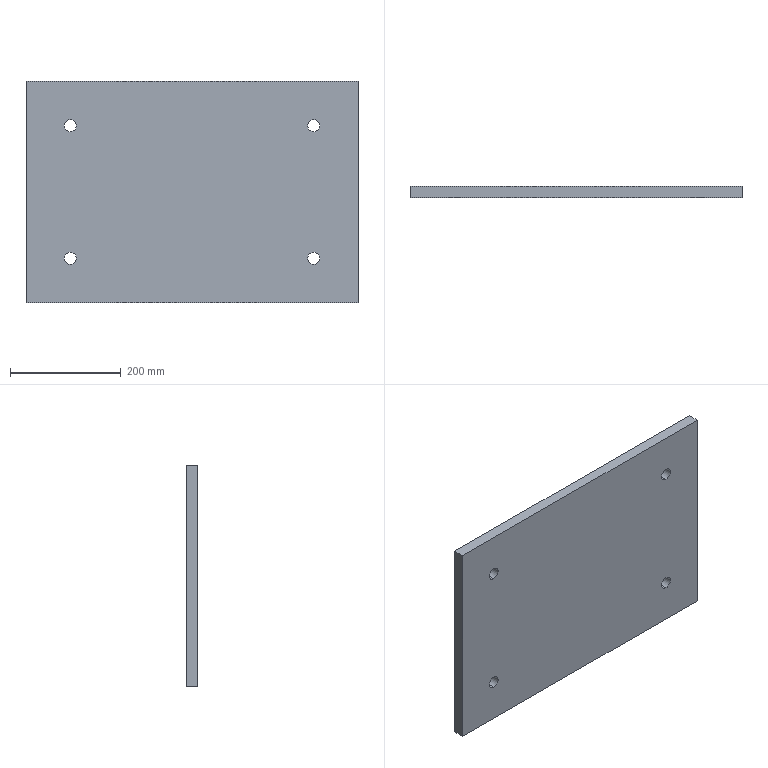Part | SolidWorks | features Extrusion 1, ICE 1 | 1 solid | 14 faces | box 600 x 20 x 400 mm | volume 4769589 mm3 | cylinder 8 | plane 6 | commonest cylinder face diameters 22 x8
STEP:
#1=CARTESIAN_POINT('',(-220.,0.,109.));
#2=VERTEX_POINT('',#1);
#3=CARTESIAN_POINT('',(-220.,0.,131.));
#4=VERTEX_POINT('',#3);
#5=CARTESIAN_POINT('',(-220.,0.,120.));
#6=DIRECTION('',(0.,1.,0.));
#7=DIRECTION('',(0.,0.,-1.));
#8=AXIS2_PLACEMENT_3D('',#5,#6,#7);
#9=CIRCLE('',#8,11.);
#10=EDGE_CURVE('',#2,#4,#9,.T.);
#11=ORIENTED_EDGE('',*,*,#10,.F.);
#12=CARTESIAN_POINT('',(-220.,20.,109.));
#13=VERTEX_POINT('',#12);
#14=CARTESIAN_POINT('',(-220.,0.,109.));
#15=DIRECTION('',(0.,1.,0.));
#16=VECTOR('',#15,1000.);
#17=LINE('',#14,#16);
#18=EDGE_CURVE('',#2,#13,#17,.T.);
#19=ORIENTED_EDGE('',*,*,#18,.T.);
#20=CARTESIAN_POINT('',(-220.,20.,131.));
#21=VERTEX_POINT('',#20);
#22=CARTESIAN_POINT('',(-220.,20.,120.));
#23=DIRECTION('',(0.,1.,0.));
#24=DIRECTION('',(0.,0.,-1.));
#25=AXIS2_PLACEMENT_3D('',#22,#23,#24);
#26=CIRCLE('',#25,11.);
#27=EDGE_CURVE('',#13,#21,#26,.T.);
#28=ORIENTED_EDGE('',*,*,#27,.T.);
#29=CARTESIAN_POINT('',(-220.,0.,131.));
#30=DIRECTION('',(0.,1.,0.));
#31=VECTOR('',#30,1000.);
#32=LINE('',#29,#31);
#33=EDGE_CURVE('',#4,#21,#32,.T.);
#34=ORIENTED_EDGE('',*,*,#33,.F.);
#35=EDGE_LOOP('',(#11,#19,#28,#34));
#36=FACE_OUTER_BOUND('',#35,.T.);
#37=CARTESIAN_POINT('',(-220.,0.,120.));
#38=DIRECTION('',(0.,1.,0.));
#39=DIRECTION('',(0.,0.,1.));
#40=AXIS2_PLACEMENT_3D('',#37,#38,#39);
#41=CYLINDRICAL_SURFACE('',#40,11.);
#42=ADVANCED_FACE('',(#36),#41,.F.);
#43=CARTESIAN_POINT('',(220.,0.,109.));
#44=VERTEX_POINT('',#43);
#45=CARTESIAN_POINT('',(220.,0.,131.));
#46=VERTEX_POINT('',#45);
#47=CARTESIAN_POINT('',(220.,0.,120.));
#48=DIRECTION('',(0.,1.,0.));
#49=DIRECTION('',(0.,0.,1.));
#50=AXIS2_PLACEMENT_3D('',#47,#48,#49);
#51=CIRCLE('',#50,11.);
#52=EDGE_CURVE('',#44,#46,#51,.T.);
#53=ORIENTED_EDGE('',*,*,#52,.F.);
#54=CARTESIAN_POINT('',(220.,20.,109.));
#55=VERTEX_POINT('',#54);
#56=CARTESIAN_POINT('',(220.,0.,109.));
#57=DIRECTION('',(0.,1.,0.));
#58=VECTOR('',#57,1000.);
#59=LINE('',#56,#58);
#60=EDGE_CURVE('',#44,#55,#59,.T.);
#61=ORIENTED_EDGE('',*,*,#60,.T.);
#62=CARTESIAN_POINT('',(220.,20.,131.));
#63=VERTEX_POINT('',#62);
#64=CARTESIAN_POINT('',(220.,20.,120.));
#65=DIRECTION('',(0.,1.,0.));
#66=DIRECTION('',(0.,0.,1.));
#67=AXIS2_PLACEMENT_3D('',#64,#65,#66);
#68=CIRCLE('',#67,11.);
#69=EDGE_CURVE('',#55,#63,#68,.T.);
#70=ORIENTED_EDGE('',*,*,#69,.T.);
#71=CARTESIAN_POINT('',(220.,0.,131.));
#72=DIRECTION('',(0.,1.,0.));
#73=VECTOR('',#72,1000.);
#74=LINE('',#71,#73);
#75=EDGE_CURVE('',#46,#63,#74,.T.);
#76=ORIENTED_EDGE('',*,*,#75,.F.);
#77=EDGE_LOOP('',(#53,#61,#70,#76));
#78=FACE_OUTER_BOUND('',#77,.T.);
#79=CARTESIAN_POINT('',(220.,0.,120.));
#80=DIRECTION('',(0.,1.,0.));
#81=DIRECTION('',(0.,0.,1.));
#82=AXIS2_PLACEMENT_3D('',#79,#80,#81);
#83=CYLINDRICAL_SURFACE('',#82,11.);
#84=ADVANCED_FACE('',(#78),#83,.F.);
#85=CARTESIAN_POINT('',(220.,0.,-131.));
#86=VERTEX_POINT('',#85);
#87=CARTESIAN_POINT('',(220.,0.,-109.));
#88=VERTEX_POINT('',#87);
#89=CARTESIAN_POINT('',(220.,0.,-120.));
#90=DIRECTION('',(0.,1.,0.));
#91=DIRECTION('',(0.,0.,-1.));
#92=AXIS2_PLACEMENT_3D('',#89,#90,#91);
#93=CIRCLE('',#92,11.);
#94=EDGE_CURVE('',#86,#88,#93,.T.);
#95=ORIENTED_EDGE('',*,*,#94,.F.);
#96=CARTESIAN_POINT('',(220.,20.,-131.));
#97=VERTEX_POINT('',#96);
#98=CARTESIAN_POINT('',(220.,0.,-131.));
#99=DIRECTION('',(0.,1.,0.));
#100=VECTOR('',#99,1000.);
#101=LINE('',#98,#100);
#102=EDGE_CURVE('',#86,#97,#101,.T.);
#103=ORIENTED_EDGE('',*,*,#102,.T.);
#104=CARTESIAN_POINT('',(220.,20.,-109.));
#105=VERTEX_POINT('',#104);
#106=CARTESIAN_POINT('',(220.,20.,-120.));
#107=DIRECTION('',(0.,1.,0.));
#108=DIRECTION('',(0.,0.,-1.));
#109=AXIS2_PLACEMENT_3D('',#106,#107,#108);
#110=CIRCLE('',#109,11.);
#111=EDGE_CURVE('',#97,#105,#110,.T.);
#112=ORIENTED_EDGE('',*,*,#111,.T.);
#113=CARTESIAN_POINT('',(220.,0.,-109.));
#114=DIRECTION('',(0.,1.,0.));
#115=VECTOR('',#114,1000.);
#116=LINE('',#113,#115);
#117=EDGE_CURVE('',#88,#105,#116,.T.);
#118=ORIENTED_EDGE('',*,*,#117,.F.);
#119=EDGE_LOOP('',(#95,#103,#112,#118));
#120=FACE_OUTER_BOUND('',#119,.T.);
#121=CARTESIAN_POINT('',(220.,0.,-120.));
#122=DIRECTION('',(0.,1.,0.));
#123=DIRECTION('',(0.,0.,1.));
#124=AXIS2_PLACEMENT_3D('',#121,#122,#123);
#125=CYLINDRICAL_SURFACE('',#124,11.);
#126=ADVANCED_FACE('',(#120),#125,.F.);
#127=CARTESIAN_POINT('',(-220.,0.,-131.));
#128=VERTEX_POINT('',#127);
#129=CARTESIAN_POINT('',(-220.,0.,-109.));
#130=VERTEX_POINT('',#129);
#131=CARTESIAN_POINT('',(-220.,0.,-120.));
#132=DIRECTION('',(0.,1.,0.));
#133=DIRECTION('',(0.,0.,1.));
#134=AXIS2_PLACEMENT_3D('',#131,#132,#133);
#135=CIRCLE('',#134,11.);
#136=EDGE_CURVE('',#128,#130,#135,.T.);
#137=ORIENTED_EDGE('',*,*,#136,.F.);
#138=CARTESIAN_POINT('',(-220.,20.,-131.));
#139=VERTEX_POINT('',#138);
#140=CARTESIAN_POINT('',(-220.,0.,-131.));
#141=DIRECTION('',(0.,1.,0.));
#142=VECTOR('',#141,1000.);
#143=LINE('',#140,#142);
#144=EDGE_CURVE('',#128,#139,#143,.T.);
#145=ORIENTED_EDGE('',*,*,#144,.T.);
#146=CARTESIAN_POINT('',(-220.,20.,-109.));
#147=VERTEX_POINT('',#146);
#148=CARTESIAN_POINT('',(-220.,20.,-120.));
#149=DIRECTION('',(0.,1.,0.));
#150=DIRECTION('',(0.,0.,1.));
#151=AXIS2_PLACEMENT_3D('',#148,#149,#150);
#152=CIRCLE('',#151,11.);
#153=EDGE_CURVE('',#139,#147,#152,.T.);
#154=ORIENTED_EDGE('',*,*,#153,.T.);
#155=CARTESIAN_POINT('',(-220.,0.,-109.));
#156=DIRECTION('',(0.,1.,0.));
#157=VECTOR('',#156,1000.);
#158=LINE('',#155,#157);
#159=EDGE_CURVE('',#130,#147,#158,.T.);
#160=ORIENTED_EDGE('',*,*,#159,.F.);
#161=EDGE_LOOP('',(#137,#145,#154,#160));
#162=FACE_OUTER_BOUND('',#161,.T.);
#163=CARTESIAN_POINT('',(-220.,0.,-120.));
#164=DIRECTION('',(0.,1.,0.));
#165=DIRECTION('',(0.,0.,1.));
#166=AXIS2_PLACEMENT_3D('',#163,#164,#165);
#167=CYLINDRICAL_SURFACE('',#166,11.);
#168=ADVANCED_FACE('',(#162),#167,.F.);
#169=CARTESIAN_POINT('',(300.,0.,200.));
#170=VERTEX_POINT('',#169);
#171=CARTESIAN_POINT('',(300.,0.,-200.));
#172=VERTEX_POINT('',#171);
#173=CARTESIAN_POINT('',(300.,0.,200.));
#174=DIRECTION('',(0.,0.,-1.));
#175=VECTOR('',#174,1000.);
#176=LINE('',#173,#175);
#177=EDGE_CURVE('',#170,#172,#176,.T.);
#178=ORIENTED_EDGE('',*,*,#177,.T.);
#179=CARTESIAN_POINT('',(300.,20.,-200.));
#180=VERTEX_POINT('',#179);
#181=CARTESIAN_POINT('',(300.,20.,-200.));
#182=DIRECTION('',(0.,-1.,0.));
#183=VECTOR('',#182,1000.);
#184=LINE('',#181,#183);
#185=EDGE_CURVE('',#180,#172,#184,.T.);
#186=ORIENTED_EDGE('',*,*,#185,.F.);
#187=CARTESIAN_POINT('',(300.,20.,200.));
#188=VERTEX_POINT('',#187);
#189=CARTESIAN_POINT('',(300.,20.,200.));
#190=DIRECTION('',(0.,0.,-1.));
#191=VECTOR('',#190,1000.);
#192=LINE('',#189,#191);
#193=EDGE_CURVE('',#188,#180,#192,.T.);
#194=ORIENTED_EDGE('',*,*,#193,.F.);
#195=CARTESIAN_POINT('',(300.,20.,200.));
#196=DIRECTION('',(0.,-1.,0.));
#197=VECTOR('',#196,1000.);
#198=LINE('',#195,#197);
#199=EDGE_CURVE('',#188,#170,#198,.T.);
#200=ORIENTED_EDGE('',*,*,#199,.T.);
#201=EDGE_LOOP('',(#178,#186,#194,#200));
#202=FACE_OUTER_BOUND('',#201,.T.);
#203=CARTESIAN_POINT('',(300.,20.,200.));
#204=DIRECTION('',(-1.,0.,0.));
#205=DIRECTION('',(0.,0.,1.));
#206=AXIS2_PLACEMENT_3D('',#203,#204,#205);
#207=PLANE('',#206);
#208=ADVANCED_FACE('',(#202),#207,.F.);
#209=CARTESIAN_POINT('',(-300.,0.,-200.));
#210=VERTEX_POINT('',#209);
#211=CARTESIAN_POINT('',(-300.,0.,-200.));
#212=DIRECTION('',(-1.,0.,0.));
#213=VECTOR('',#212,1000.);
#214=LINE('',#211,#213);
#215=EDGE_CURVE('',#172,#210,#214,.T.);
#216=ORIENTED_EDGE('',*,*,#215,.T.);
#217=CARTESIAN_POINT('',(-300.,20.,-200.));
#218=VERTEX_POINT('',#217);
#219=CARTESIAN_POINT('',(-300.,20.,-200.));
#220=DIRECTION('',(0.,-1.,0.));
#221=VECTOR('',#220,1000.);
#222=LINE('',#219,#221);
#223=EDGE_CURVE('',#218,#210,#222,.T.);
#224=ORIENTED_EDGE('',*,*,#223,.F.);
#225=CARTESIAN_POINT('',(-300.,20.,-200.));
#226=DIRECTION('',(-1.,0.,0.));
#227=VECTOR('',#226,1000.);
#228=LINE('',#225,#227);
#229=EDGE_CURVE('',#180,#218,#228,.T.);
#230=ORIENTED_EDGE('',*,*,#229,.F.);
#231=ORIENTED_EDGE('',*,*,#185,.T.);
#232=EDGE_LOOP('',(#216,#224,#230,#231));
#233=FACE_OUTER_BOUND('',#232,.T.);
#234=CARTESIAN_POINT('',(-300.,20.,-200.));
#235=DIRECTION('',(0.,0.,1.));
#236=DIRECTION('',(1.,0.,0.));
#237=AXIS2_PLACEMENT_3D('',#234,#235,#236);
#238=PLANE('',#237);
#239=ADVANCED_FACE('',(#233),#238,.F.);
#240=CARTESIAN_POINT('',(-300.,0.,200.));
#241=VERTEX_POINT('',#240);
#242=CARTESIAN_POINT('',(-300.,0.,200.));
#243=DIRECTION('',(0.,0.,1.));
#244=VECTOR('',#243,1000.);
#245=LINE('',#242,#244);
#246=EDGE_CURVE('',#210,#241,#245,.T.);
#247=ORIENTED_EDGE('',*,*,#246,.T.);
#248=CARTESIAN_POINT('',(-300.,20.,200.));
#249=VERTEX_POINT('',#248);
#250=CARTESIAN_POINT('',(-300.,20.,200.));
#251=DIRECTION('',(0.,-1.,0.));
#252=VECTOR('',#251,1000.);
#253=LINE('',#250,#252);
#254=EDGE_CURVE('',#249,#241,#253,.T.);
#255=ORIENTED_EDGE('',*,*,#254,.F.);
#256=CARTESIAN_POINT('',(-300.,20.,200.));
#257=DIRECTION('',(0.,0.,1.));
#258=VECTOR('',#257,1000.);
#259=LINE('',#256,#258);
#260=EDGE_CURVE('',#218,#249,#259,.T.);
#261=ORIENTED_EDGE('',*,*,#260,.F.);
#262=ORIENTED_EDGE('',*,*,#223,.T.);
#263=EDGE_LOOP('',(#247,#255,#261,#262));
#264=FACE_OUTER_BOUND('',#263,.T.);
#265=CARTESIAN_POINT('',(-300.,20.,200.));
#266=DIRECTION('',(1.,0.,0.));
#267=DIRECTION('',(0.,0.,-1.));
#268=AXIS2_PLACEMENT_3D('',#265,#266,#267);
#269=PLANE('',#268);
#270=ADVANCED_FACE('',(#264),#269,.F.);
#271=CARTESIAN_POINT('',(-300.,0.,200.));
#272=DIRECTION('',(1.,0.,0.));
#273=VECTOR('',#272,1000.);
#274=LINE('',#271,#273);
#275=EDGE_CURVE('',#241,#170,#274,.T.);
#276=ORIENTED_EDGE('',*,*,#275,.T.);
#277=ORIENTED_EDGE('',*,*,#199,.F.);
#278=CARTESIAN_POINT('',(-300.,20.,200.));
#279=DIRECTION('',(1.,0.,0.));
#280=VECTOR('',#279,1000.);
#281=LINE('',#278,#280);
#282=EDGE_CURVE('',#249,#188,#281,.T.);
#283=ORIENTED_EDGE('',*,*,#282,.F.);
#284=ORIENTED_EDGE('',*,*,#254,.T.);
#285=EDGE_LOOP('',(#276,#277,#283,#284));
#286=FACE_OUTER_BOUND('',#285,.T.);
#287=CARTESIAN_POINT('',(-300.,20.,200.));
#288=DIRECTION('',(0.,0.,-1.));
#289=DIRECTION('',(-1.,0.,0.));
#290=AXIS2_PLACEMENT_3D('',#287,#288,#289);
#291=PLANE('',#290);
#292=ADVANCED_FACE('',(#286),#291,.F.);
#293=CARTESIAN_POINT('',(-220.,20.,120.));
#294=DIRECTION('',(0.,1.,0.));
#295=DIRECTION('',(0.,0.,-1.));
#296=AXIS2_PLACEMENT_3D('',#293,#294,#295);
#297=CIRCLE('',#296,11.);
#298=EDGE_CURVE('',#21,#13,#297,.T.);
#299=ORIENTED_EDGE('',*,*,#298,.F.);
#300=ORIENTED_EDGE('',*,*,#27,.F.);
#301=EDGE_LOOP('',(#299,#300));
#302=FACE_BOUND('',#301,.T.);
#303=CARTESIAN_POINT('',(220.,20.,120.));
#304=DIRECTION('',(0.,1.,0.));
#305=DIRECTION('',(0.,0.,1.));
#306=AXIS2_PLACEMENT_3D('',#303,#304,#305);
#307=CIRCLE('',#306,11.);
#308=EDGE_CURVE('',#63,#55,#307,.T.);
#309=ORIENTED_EDGE('',*,*,#308,.F.);
#310=ORIENTED_EDGE('',*,*,#69,.F.);
#311=EDGE_LOOP('',(#309,#310));
#312=FACE_BOUND('',#311,.T.);
#313=CARTESIAN_POINT('',(220.,20.,-120.));
#314=DIRECTION('',(0.,1.,0.));
#315=DIRECTION('',(0.,0.,-1.));
#316=AXIS2_PLACEMENT_3D('',#313,#314,#315);
#317=CIRCLE('',#316,11.);
#318=EDGE_CURVE('',#105,#97,#317,.T.);
#319=ORIENTED_EDGE('',*,*,#318,.F.);
#320=ORIENTED_EDGE('',*,*,#111,.F.);
#321=EDGE_LOOP('',(#319,#320));
#322=FACE_BOUND('',#321,.T.);
#323=CARTESIAN_POINT('',(-220.,20.,-120.));
#324=DIRECTION('',(0.,1.,0.));
#325=DIRECTION('',(0.,0.,1.));
#326=AXIS2_PLACEMENT_3D('',#323,#324,#325);
#327=CIRCLE('',#326,11.);
#328=EDGE_CURVE('',#147,#139,#327,.T.);
#329=ORIENTED_EDGE('',*,*,#328,.F.);
#330=ORIENTED_EDGE('',*,*,#153,.F.);
#331=EDGE_LOOP('',(#329,#330));
#332=FACE_BOUND('',#331,.T.);
#333=ORIENTED_EDGE('',*,*,#193,.T.);
#334=ORIENTED_EDGE('',*,*,#229,.T.);
#335=ORIENTED_EDGE('',*,*,#260,.T.);
#336=ORIENTED_EDGE('',*,*,#282,.T.);
#337=EDGE_LOOP('',(#333,#334,#335,#336));
#338=FACE_OUTER_BOUND('',#337,.T.);
#339=CARTESIAN_POINT('',(0.,20.,0.));
#340=DIRECTION('',(0.,-1.,0.));
#341=DIRECTION('',(0.,0.,-1.));
#342=AXIS2_PLACEMENT_3D('',#339,#340,#341);
#343=PLANE('',#342);
#344=ADVANCED_FACE('',(#302,#312,#322,#332,#338),#343,.F.);
#345=CARTESIAN_POINT('',(-220.,0.,120.));
#346=DIRECTION('',(0.,1.,0.));
#347=DIRECTION('',(0.,0.,-1.));
#348=AXIS2_PLACEMENT_3D('',#345,#346,#347);
#349=CIRCLE('',#348,11.);
#350=EDGE_CURVE('',#4,#2,#349,.T.);
#351=ORIENTED_EDGE('',*,*,#350,.T.);
#352=ORIENTED_EDGE('',*,*,#10,.T.);
#353=EDGE_LOOP('',(#351,#352));
#354=FACE_BOUND('',#353,.T.);
#355=CARTESIAN_POINT('',(220.,0.,120.));
#356=DIRECTION('',(0.,1.,0.));
#357=DIRECTION('',(0.,0.,1.));
#358=AXIS2_PLACEMENT_3D('',#355,#356,#357);
#359=CIRCLE('',#358,11.);
#360=EDGE_CURVE('',#46,#44,#359,.T.);
#361=ORIENTED_EDGE('',*,*,#360,.T.);
#362=ORIENTED_EDGE('',*,*,#52,.T.);
#363=EDGE_LOOP('',(#361,#362));
#364=FACE_BOUND('',#363,.T.);
#365=CARTESIAN_POINT('',(220.,0.,-120.));
#366=DIRECTION('',(0.,1.,0.));
#367=DIRECTION('',(0.,0.,-1.));
#368=AXIS2_PLACEMENT_3D('',#365,#366,#367);
#369=CIRCLE('',#368,11.);
#370=EDGE_CURVE('',#88,#86,#369,.T.);
#371=ORIENTED_EDGE('',*,*,#370,.T.);
#372=ORIENTED_EDGE('',*,*,#94,.T.);
#373=EDGE_LOOP('',(#371,#372));
#374=FACE_BOUND('',#373,.T.);
#375=CARTESIAN_POINT('',(-220.,0.,-120.));
#376=DIRECTION('',(0.,1.,0.));
#377=DIRECTION('',(0.,0.,1.));
#378=AXIS2_PLACEMENT_3D('',#375,#376,#377);
#379=CIRCLE('',#378,11.);
#380=EDGE_CURVE('',#130,#128,#379,.T.);
#381=ORIENTED_EDGE('',*,*,#380,.T.);
#382=ORIENTED_EDGE('',*,*,#136,.T.);
#383=EDGE_LOOP('',(#381,#382));
#384=FACE_BOUND('',#383,.T.);
#385=ORIENTED_EDGE('',*,*,#177,.F.);
#386=ORIENTED_EDGE('',*,*,#275,.F.);
#387=ORIENTED_EDGE('',*,*,#246,.F.);
#388=ORIENTED_EDGE('',*,*,#215,.F.);
#389=EDGE_LOOP('',(#385,#386,#387,#388));
#390=FACE_OUTER_BOUND('',#389,.T.);
#391=CARTESIAN_POINT('',(0.,0.,0.));
#392=DIRECTION('',(0.,-1.,0.));
#393=DIRECTION('',(0.,0.,-1.));
#394=AXIS2_PLACEMENT_3D('',#391,#392,#393);
#395=PLANE('',#394);
#396=ADVANCED_FACE('',(#354,#364,#374,#384,#390),#395,.T.);
#397=ORIENTED_EDGE('',*,*,#144,.F.);
#398=ORIENTED_EDGE('',*,*,#380,.F.);
#399=ORIENTED_EDGE('',*,*,#159,.T.);
#400=ORIENTED_EDGE('',*,*,#328,.T.);
#401=EDGE_LOOP('',(#397,#398,#399,#400));
#402=FACE_OUTER_BOUND('',#401,.T.);
#403=CARTESIAN_POINT('',(-220.,0.,-120.));
#404=DIRECTION('',(0.,1.,0.));
#405=DIRECTION('',(0.,0.,1.));
#406=AXIS2_PLACEMENT_3D('',#403,#404,#405);
#407=CYLINDRICAL_SURFACE('',#406,11.);
#408=ADVANCED_FACE('',(#402),#407,.F.);
#409=ORIENTED_EDGE('',*,*,#102,.F.);
#410=ORIENTED_EDGE('',*,*,#370,.F.);
#411=ORIENTED_EDGE('',*,*,#117,.T.);
#412=ORIENTED_EDGE('',*,*,#318,.T.);
#413=EDGE_LOOP('',(#409,#410,#411,#412));
#414=FACE_OUTER_BOUND('',#413,.T.);
#415=CARTESIAN_POINT('',(220.,0.,-120.));
#416=DIRECTION('',(0.,1.,0.));
#417=DIRECTION('',(0.,0.,1.));
#418=AXIS2_PLACEMENT_3D('',#415,#416,#417);
#419=CYLINDRICAL_SURFACE('',#418,11.);
#420=ADVANCED_FACE('',(#414),#419,.F.);
#421=ORIENTED_EDGE('',*,*,#60,.F.);
#422=ORIENTED_EDGE('',*,*,#360,.F.);
#423=ORIENTED_EDGE('',*,*,#75,.T.);
#424=ORIENTED_EDGE('',*,*,#308,.T.);
#425=EDGE_LOOP('',(#421,#422,#423,#424));
#426=FACE_OUTER_BOUND('',#425,.T.);
#427=CARTESIAN_POINT('',(220.,0.,120.));
#428=DIRECTION('',(0.,1.,0.));
#429=DIRECTION('',(0.,0.,1.));
#430=AXIS2_PLACEMENT_3D('',#427,#428,#429);
#431=CYLINDRICAL_SURFACE('',#430,11.);
#432=ADVANCED_FACE('',(#426),#431,.F.);
#433=ORIENTED_EDGE('',*,*,#18,.F.);
#434=ORIENTED_EDGE('',*,*,#350,.F.);
#435=ORIENTED_EDGE('',*,*,#33,.T.);
#436=ORIENTED_EDGE('',*,*,#298,.T.);
#437=EDGE_LOOP('',(#433,#434,#435,#436));
#438=FACE_OUTER_BOUND('',#437,.T.);
#439=CARTESIAN_POINT('',(-220.,0.,120.));
#440=DIRECTION('',(0.,1.,0.));
#441=DIRECTION('',(0.,0.,1.));
#442=AXIS2_PLACEMENT_3D('',#439,#440,#441);
#443=CYLINDRICAL_SURFACE('',#442,11.);
#444=ADVANCED_FACE('',(#438),#443,.F.);
#445=CLOSED_SHELL('',(#42,#84,#126,#168,#208,#239,#270,#292,#344,#396,#408,#420,#432,#444));
#446=MANIFOLD_SOLID_BREP('',#445);
#447=CARTESIAN_POINT('',(0.,0.,0.));
#448=DIRECTION('',(0.,0.,1.));
#449=DIRECTION('',(1.,0.,0.));
#450=AXIS2_PLACEMENT_3D('',#447,#448,#449);
#451=(LENGTH_UNIT()NAMED_UNIT(*)SI_UNIT(.MILLI.,.METRE.));
#452=UNCERTAINTY_MEASURE_WITH_UNIT(LENGTH_MEASURE(0.00001),#451,'','');
#453=(NAMED_UNIT(*)PLANE_ANGLE_UNIT()SI_UNIT($,.RADIAN.));
#454=(NAMED_UNIT(*)SI_UNIT($,.STERADIAN.)SOLID_ANGLE_UNIT());
#455=(GEOMETRIC_REPRESENTATION_CONTEXT(3)GLOBAL_UNCERTAINTY_ASSIGNED_CONTEXT((#452))GLOBAL_UNIT_ASSIGNED_CONTEXT((#451,#453,#454))REPRESENTATION_CONTEXT('',''));
#456=ADVANCED_BREP_SHAPE_REPRESENTATION('',(#446,#450),#455);